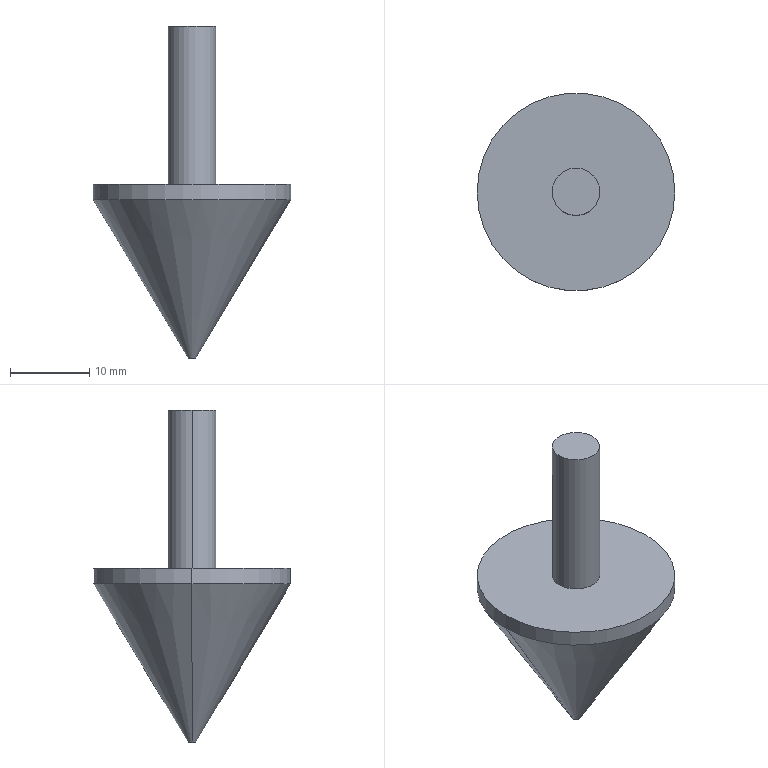Part | SolidWorks | features Extrusion 1, ICE 1, Revolution 1 | 1 solid | 9 faces | box 25 x 25 x 42 mm | volume 4956 mm3 | cylinder 4 | plane 3 | cone 2 | commonest cylinder face diameters 6 x2 25 x2
STEP:
#1=CARTESIAN_POINT('',(-0.5,0.,-22.));
#2=VERTEX_POINT('',#1);
#3=CARTESIAN_POINT('',(0.5,0.,-22.));
#4=VERTEX_POINT('',#3);
#5=CARTESIAN_POINT('',(0.,0.,-22.));
#6=DIRECTION('',(0.,0.,-1.));
#7=DIRECTION('',(-1.,0.,0.));
#8=AXIS2_PLACEMENT_3D('',#5,#6,#7);
#9=CIRCLE('',#8,0.5);
#10=EDGE_CURVE('',#2,#4,#9,.T.);
#11=ORIENTED_EDGE('',*,*,#10,.F.);
#12=CARTESIAN_POINT('',(-12.5,0.,-2.));
#13=VERTEX_POINT('',#12);
#14=CARTESIAN_POINT('',(-0.5,0.,-22.));
#15=DIRECTION('',(-0.5145,0.,0.8575));
#16=VECTOR('',#15,1000.);
#17=LINE('',#14,#16);
#18=EDGE_CURVE('',#2,#13,#17,.T.);
#19=ORIENTED_EDGE('',*,*,#18,.T.);
#20=CARTESIAN_POINT('',(12.5,0.,-2.));
#21=VERTEX_POINT('',#20);
#22=CARTESIAN_POINT('',(0.,0.,-2.));
#23=DIRECTION('',(0.,0.,-1.));
#24=DIRECTION('',(-1.,0.,0.));
#25=AXIS2_PLACEMENT_3D('',#22,#23,#24);
#26=CIRCLE('',#25,12.5);
#27=EDGE_CURVE('',#13,#21,#26,.T.);
#28=ORIENTED_EDGE('',*,*,#27,.T.);
#29=CARTESIAN_POINT('',(0.5,0.,-22.));
#30=DIRECTION('',(0.5145,0.,0.8575));
#31=VECTOR('',#30,1000.);
#32=LINE('',#29,#31);
#33=EDGE_CURVE('',#4,#21,#32,.T.);
#34=ORIENTED_EDGE('',*,*,#33,.F.);
#35=EDGE_LOOP('',(#11,#19,#28,#34));
#36=FACE_OUTER_BOUND('',#35,.T.);
#37=CARTESIAN_POINT('',(0.,0.,-22.));
#38=DIRECTION('',(0.,0.,1.));
#39=DIRECTION('',(1.,0.,0.));
#40=AXIS2_PLACEMENT_3D('',#37,#38,#39);
#41=CONICAL_SURFACE('',#40,0.5,0.5404);
#42=ADVANCED_FACE('',(#36),#41,.T.);
#43=ORIENTED_EDGE('',*,*,#27,.F.);
#44=CARTESIAN_POINT('',(-12.5,0.,0.));
#45=VERTEX_POINT('',#44);
#46=CARTESIAN_POINT('',(-12.5,0.,-2.));
#47=DIRECTION('',(0.,0.,1.));
#48=VECTOR('',#47,1000.);
#49=LINE('',#46,#48);
#50=EDGE_CURVE('',#13,#45,#49,.T.);
#51=ORIENTED_EDGE('',*,*,#50,.T.);
#52=CARTESIAN_POINT('',(12.5,0.,0.));
#53=VERTEX_POINT('',#52);
#54=CARTESIAN_POINT('',(0.,0.,0.));
#55=DIRECTION('',(0.,0.,-1.));
#56=DIRECTION('',(-1.,0.,0.));
#57=AXIS2_PLACEMENT_3D('',#54,#55,#56);
#58=CIRCLE('',#57,12.5);
#59=EDGE_CURVE('',#45,#53,#58,.T.);
#60=ORIENTED_EDGE('',*,*,#59,.T.);
#61=CARTESIAN_POINT('',(12.5,0.,-2.));
#62=DIRECTION('',(0.,0.,1.));
#63=VECTOR('',#62,1000.);
#64=LINE('',#61,#63);
#65=EDGE_CURVE('',#21,#53,#64,.T.);
#66=ORIENTED_EDGE('',*,*,#65,.F.);
#67=EDGE_LOOP('',(#43,#51,#60,#66));
#68=FACE_OUTER_BOUND('',#67,.T.);
#69=CARTESIAN_POINT('',(0.,0.,-2.));
#70=DIRECTION('',(0.,0.,1.));
#71=DIRECTION('',(1.,0.,0.));
#72=AXIS2_PLACEMENT_3D('',#69,#70,#71);
#73=CYLINDRICAL_SURFACE('',#72,12.5);
#74=ADVANCED_FACE('',(#68),#73,.T.);
#75=CARTESIAN_POINT('',(3.,0.,20.));
#76=VERTEX_POINT('',#75);
#77=CARTESIAN_POINT('',(-3.,0.,20.));
#78=VERTEX_POINT('',#77);
#79=CARTESIAN_POINT('',(0.,0.,20.));
#80=DIRECTION('',(0.,0.,1.));
#81=DIRECTION('',(1.,0.,0.));
#82=AXIS2_PLACEMENT_3D('',#79,#80,#81);
#83=CIRCLE('',#82,3.);
#84=EDGE_CURVE('',#76,#78,#83,.T.);
#85=ORIENTED_EDGE('',*,*,#84,.F.);
#86=CARTESIAN_POINT('',(3.,0.,0.));
#87=VERTEX_POINT('',#86);
#88=CARTESIAN_POINT('',(3.,0.,20.));
#89=DIRECTION('',(0.,0.,-1.));
#90=VECTOR('',#89,1000.);
#91=LINE('',#88,#90);
#92=EDGE_CURVE('',#76,#87,#91,.T.);
#93=ORIENTED_EDGE('',*,*,#92,.T.);
#94=CARTESIAN_POINT('',(-3.,0.,0.));
#95=VERTEX_POINT('',#94);
#96=CARTESIAN_POINT('',(0.,0.,0.));
#97=DIRECTION('',(0.,0.,1.));
#98=DIRECTION('',(1.,0.,0.));
#99=AXIS2_PLACEMENT_3D('',#96,#97,#98);
#100=CIRCLE('',#99,3.);
#101=EDGE_CURVE('',#87,#95,#100,.T.);
#102=ORIENTED_EDGE('',*,*,#101,.T.);
#103=CARTESIAN_POINT('',(-3.,0.,20.));
#104=DIRECTION('',(0.,0.,-1.));
#105=VECTOR('',#104,1000.);
#106=LINE('',#103,#105);
#107=EDGE_CURVE('',#78,#95,#106,.T.);
#108=ORIENTED_EDGE('',*,*,#107,.F.);
#109=EDGE_LOOP('',(#85,#93,#102,#108));
#110=FACE_OUTER_BOUND('',#109,.T.);
#111=CARTESIAN_POINT('',(0.,0.,20.));
#112=DIRECTION('',(0.,0.,-1.));
#113=DIRECTION('',(-1.,0.,0.));
#114=AXIS2_PLACEMENT_3D('',#111,#112,#113);
#115=CYLINDRICAL_SURFACE('',#114,3.);
#116=ADVANCED_FACE('',(#110),#115,.T.);
#117=ORIENTED_EDGE('',*,*,#92,.F.);
#118=CARTESIAN_POINT('',(0.,0.,20.));
#119=DIRECTION('',(0.,0.,1.));
#120=DIRECTION('',(1.,0.,0.));
#121=AXIS2_PLACEMENT_3D('',#118,#119,#120);
#122=CIRCLE('',#121,3.);
#123=EDGE_CURVE('',#78,#76,#122,.T.);
#124=ORIENTED_EDGE('',*,*,#123,.F.);
#125=ORIENTED_EDGE('',*,*,#107,.T.);
#126=CARTESIAN_POINT('',(0.,0.,0.));
#127=DIRECTION('',(0.,0.,1.));
#128=DIRECTION('',(1.,0.,0.));
#129=AXIS2_PLACEMENT_3D('',#126,#127,#128);
#130=CIRCLE('',#129,3.);
#131=EDGE_CURVE('',#95,#87,#130,.T.);
#132=ORIENTED_EDGE('',*,*,#131,.T.);
#133=EDGE_LOOP('',(#117,#124,#125,#132));
#134=FACE_OUTER_BOUND('',#133,.T.);
#135=CARTESIAN_POINT('',(0.,0.,20.));
#136=DIRECTION('',(0.,0.,-1.));
#137=DIRECTION('',(-1.,0.,0.));
#138=AXIS2_PLACEMENT_3D('',#135,#136,#137);
#139=CYLINDRICAL_SURFACE('',#138,3.);
#140=ADVANCED_FACE('',(#134),#139,.T.);
#141=ORIENTED_EDGE('',*,*,#123,.T.);
#142=ORIENTED_EDGE('',*,*,#84,.T.);
#143=EDGE_LOOP('',(#141,#142));
#144=FACE_OUTER_BOUND('',#143,.T.);
#145=CARTESIAN_POINT('',(0.,0.,20.));
#146=DIRECTION('',(0.,0.,1.));
#147=DIRECTION('',(1.,0.,0.));
#148=AXIS2_PLACEMENT_3D('',#145,#146,#147);
#149=PLANE('',#148);
#150=ADVANCED_FACE('',(#144),#149,.T.);
#151=ORIENTED_EDGE('',*,*,#50,.F.);
#152=CARTESIAN_POINT('',(0.,0.,-2.));
#153=DIRECTION('',(0.,0.,-1.));
#154=DIRECTION('',(-1.,0.,0.));
#155=AXIS2_PLACEMENT_3D('',#152,#153,#154);
#156=CIRCLE('',#155,12.5);
#157=EDGE_CURVE('',#21,#13,#156,.T.);
#158=ORIENTED_EDGE('',*,*,#157,.F.);
#159=ORIENTED_EDGE('',*,*,#65,.T.);
#160=CARTESIAN_POINT('',(0.,0.,0.));
#161=DIRECTION('',(0.,0.,-1.));
#162=DIRECTION('',(-1.,0.,0.));
#163=AXIS2_PLACEMENT_3D('',#160,#161,#162);
#164=CIRCLE('',#163,12.5);
#165=EDGE_CURVE('',#53,#45,#164,.T.);
#166=ORIENTED_EDGE('',*,*,#165,.T.);
#167=EDGE_LOOP('',(#151,#158,#159,#166));
#168=FACE_OUTER_BOUND('',#167,.T.);
#169=CARTESIAN_POINT('',(0.,0.,-2.));
#170=DIRECTION('',(0.,0.,1.));
#171=DIRECTION('',(1.,0.,0.));
#172=AXIS2_PLACEMENT_3D('',#169,#170,#171);
#173=CYLINDRICAL_SURFACE('',#172,12.5);
#174=ADVANCED_FACE('',(#168),#173,.T.);
#175=ORIENTED_EDGE('',*,*,#131,.F.);
#176=ORIENTED_EDGE('',*,*,#101,.F.);
#177=EDGE_LOOP('',(#175,#176));
#178=FACE_BOUND('',#177,.T.);
#179=ORIENTED_EDGE('',*,*,#165,.F.);
#180=ORIENTED_EDGE('',*,*,#59,.F.);
#181=EDGE_LOOP('',(#179,#180));
#182=FACE_OUTER_BOUND('',#181,.T.);
#183=CARTESIAN_POINT('',(0.,0.,0.));
#184=DIRECTION('',(0.,0.,-1.));
#185=DIRECTION('',(-1.,0.,0.));
#186=AXIS2_PLACEMENT_3D('',#183,#184,#185);
#187=PLANE('',#186);
#188=ADVANCED_FACE('',(#178,#182),#187,.F.);
#189=CARTESIAN_POINT('',(0.,0.,-22.));
#190=DIRECTION('',(0.,0.,-1.));
#191=DIRECTION('',(-1.,0.,0.));
#192=AXIS2_PLACEMENT_3D('',#189,#190,#191);
#193=CIRCLE('',#192,0.5);
#194=EDGE_CURVE('',#4,#2,#193,.T.);
#195=ORIENTED_EDGE('',*,*,#194,.T.);
#196=ORIENTED_EDGE('',*,*,#10,.T.);
#197=EDGE_LOOP('',(#195,#196));
#198=FACE_OUTER_BOUND('',#197,.T.);
#199=CARTESIAN_POINT('',(-0.5,0.,-22.));
#200=DIRECTION('',(0.,0.,-1.));
#201=DIRECTION('',(-1.,0.,0.));
#202=AXIS2_PLACEMENT_3D('',#199,#200,#201);
#203=PLANE('',#202);
#204=ADVANCED_FACE('',(#198),#203,.T.);
#205=ORIENTED_EDGE('',*,*,#18,.F.);
#206=ORIENTED_EDGE('',*,*,#194,.F.);
#207=ORIENTED_EDGE('',*,*,#33,.T.);
#208=ORIENTED_EDGE('',*,*,#157,.T.);
#209=EDGE_LOOP('',(#205,#206,#207,#208));
#210=FACE_OUTER_BOUND('',#209,.T.);
#211=CARTESIAN_POINT('',(0.,0.,-22.));
#212=DIRECTION('',(0.,0.,1.));
#213=DIRECTION('',(1.,0.,0.));
#214=AXIS2_PLACEMENT_3D('',#211,#212,#213);
#215=CONICAL_SURFACE('',#214,0.5,0.5404);
#216=ADVANCED_FACE('',(#210),#215,.T.);
#217=CLOSED_SHELL('',(#42,#74,#116,#140,#150,#174,#188,#204,#216));
#218=MANIFOLD_SOLID_BREP('',#217);
#219=CARTESIAN_POINT('',(0.,0.,0.));
#220=DIRECTION('',(0.,0.,1.));
#221=DIRECTION('',(1.,0.,0.));
#222=AXIS2_PLACEMENT_3D('',#219,#220,#221);
#223=(LENGTH_UNIT()NAMED_UNIT(*)SI_UNIT(.MILLI.,.METRE.));
#224=UNCERTAINTY_MEASURE_WITH_UNIT(LENGTH_MEASURE(0.00001),#223,'','');
#225=(NAMED_UNIT(*)PLANE_ANGLE_UNIT()SI_UNIT($,.RADIAN.));
#226=(NAMED_UNIT(*)SI_UNIT($,.STERADIAN.)SOLID_ANGLE_UNIT());
#227=(GEOMETRIC_REPRESENTATION_CONTEXT(3)GLOBAL_UNCERTAINTY_ASSIGNED_CONTEXT((#224))GLOBAL_UNIT_ASSIGNED_CONTEXT((#223,#225,#226))REPRESENTATION_CONTEXT('',''));
#228=ADVANCED_BREP_SHAPE_REPRESENTATION('',(#218,#222),#227);